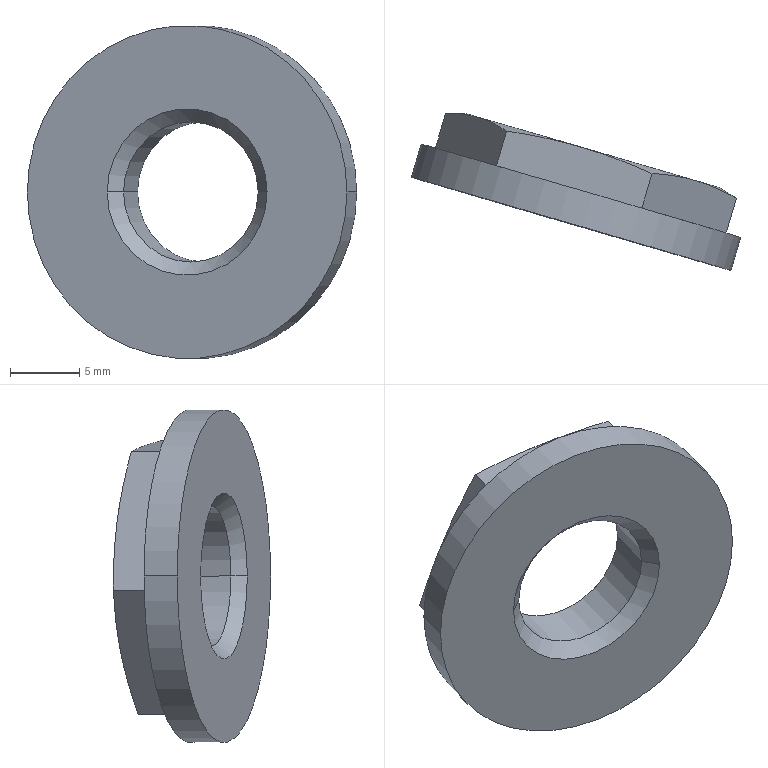Part | SolidWorks | features BaseBody 1 | 1 solid | 24 faces | box 23.74 x 11.323 x 24 mm | volume 1594 mm3 | cone 11 | plane 9 | cylinder 4 | commonest cylinder face diameters 10.106 x2 24 x2
STEP:
#1=CARTESIAN_POINT('',(-101.443,495.422,-24.879));
#2=VERTEX_POINT('',#1);
#3=CARTESIAN_POINT('',(-91.741,492.592,-24.879));
#4=VERTEX_POINT('',#3);
#5=CARTESIAN_POINT('',(-96.592,494.007,-24.879));
#6=DIRECTION('',(-0.28,-0.96,0.));
#7=DIRECTION('',(0.4011,-0.117,0.9085));
#8=AXIS2_PLACEMENT_3D('',#5,#6,#7);
#9=CIRCLE('',#8,5.053);
#10=EDGE_CURVE('',#2,#4,#9,.T.);
#11=ORIENTED_EDGE('',*,*,#10,.F.);
#12=CARTESIAN_POINT('',(-102.617,494.777,-24.879));
#13=VERTEX_POINT('',#12);
#14=CARTESIAN_POINT('',(-102.617,494.777,-24.879));
#15=DIRECTION('',(-0.8768,-0.4809,0.));
#16=VECTOR('',#15,1000.);
#17=LINE('',#14,#16);
#18=EDGE_CURVE('',#2,#13,#17,.T.);
#19=ORIENTED_EDGE('',*,*,#18,.T.);
#20=CARTESIAN_POINT('',(-91.097,491.418,-24.879));
#21=VERTEX_POINT('',#20);
#22=CARTESIAN_POINT('',(-96.857,493.098,-24.879));
#23=DIRECTION('',(0.28,0.96,0.));
#24=DIRECTION('',(0.96,-0.28,0.));
#25=AXIS2_PLACEMENT_3D('',#22,#23,#24);
#26=CIRCLE('',#25,6.);
#27=EDGE_CURVE('',#21,#13,#26,.T.);
#28=ORIENTED_EDGE('',*,*,#27,.F.);
#29=CARTESIAN_POINT('',(-91.097,491.418,-24.879));
#30=DIRECTION('',(0.4809,-0.8768,0.));
#31=VECTOR('',#30,1000.);
#32=LINE('',#29,#31);
#33=EDGE_CURVE('',#4,#21,#32,.T.);
#34=ORIENTED_EDGE('',*,*,#33,.F.);
#35=EDGE_LOOP('',(#11,#19,#28,#34));
#36=FACE_OUTER_BOUND('',#35,.T.);
#37=CARTESIAN_POINT('',(-96.857,493.098,-24.879));
#38=DIRECTION('',(-0.28,-0.96,0.));
#39=DIRECTION('',(0.96,-0.28,0.));
#40=AXIS2_PLACEMENT_3D('',#37,#38,#39);
#41=CONICAL_SURFACE('',#40,6.,0.7854);
#42=ADVANCED_FACE('',(#36),#41,.F.);
#43=CARTESIAN_POINT('',(-85.337,489.738,-24.879));
#44=VERTEX_POINT('',#43);
#45=CARTESIAN_POINT('',(-108.377,496.457,-24.879));
#46=VERTEX_POINT('',#45);
#47=CARTESIAN_POINT('',(-96.857,493.098,-24.879));
#48=DIRECTION('',(-0.28,-0.96,0.));
#49=DIRECTION('',(-0.96,0.28,0.));
#50=AXIS2_PLACEMENT_3D('',#47,#48,#49);
#51=CIRCLE('',#50,12.);
#52=EDGE_CURVE('',#44,#46,#51,.T.);
#53=ORIENTED_EDGE('',*,*,#52,.F.);
#54=CARTESIAN_POINT('',(-84.637,492.138,-24.879));
#55=VERTEX_POINT('',#54);
#56=CARTESIAN_POINT('',(-84.661,492.057,-24.879));
#57=DIRECTION('',(0.28,0.96,0.));
#58=VECTOR('',#57,1000.);
#59=LINE('',#56,#58);
#60=EDGE_CURVE('',#44,#55,#59,.T.);
#61=ORIENTED_EDGE('',*,*,#60,.T.);
#62=CARTESIAN_POINT('',(-107.677,498.857,-24.879));
#63=VERTEX_POINT('',#62);
#64=CARTESIAN_POINT('',(-96.157,495.498,-24.879));
#65=DIRECTION('',(-0.28,-0.96,0.));
#66=DIRECTION('',(-0.96,0.28,0.));
#67=AXIS2_PLACEMENT_3D('',#64,#65,#66);
#68=CIRCLE('',#67,12.);
#69=EDGE_CURVE('',#55,#63,#68,.T.);
#70=ORIENTED_EDGE('',*,*,#69,.T.);
#71=CARTESIAN_POINT('',(-107.701,498.776,-24.879));
#72=DIRECTION('',(0.28,0.96,0.));
#73=VECTOR('',#72,1000.);
#74=LINE('',#71,#73);
#75=EDGE_CURVE('',#46,#63,#74,.T.);
#76=ORIENTED_EDGE('',*,*,#75,.F.);
#77=EDGE_LOOP('',(#53,#61,#70,#76));
#78=FACE_OUTER_BOUND('',#77,.T.);
#79=CARTESIAN_POINT('',(-96.181,495.416,-24.879));
#80=DIRECTION('',(0.28,0.96,0.));
#81=DIRECTION('',(-0.96,0.28,0.));
#82=AXIS2_PLACEMENT_3D('',#79,#80,#81);
#83=CYLINDRICAL_SURFACE('',#82,12.);
#84=ADVANCED_FACE('',(#78),#83,.T.);
#85=ORIENTED_EDGE('',*,*,#10,.T.);
#86=CARTESIAN_POINT('',(-90.731,496.054,-24.879));
#87=VERTEX_POINT('',#86);
#88=CARTESIAN_POINT('',(-91.236,494.323,-24.879));
#89=DIRECTION('',(0.28,0.96,0.));
#90=VECTOR('',#89,1000.);
#91=LINE('',#88,#90);
#92=EDGE_CURVE('',#4,#87,#91,.T.);
#93=ORIENTED_EDGE('',*,*,#92,.T.);
#94=CARTESIAN_POINT('',(-100.433,498.883,-24.879));
#95=VERTEX_POINT('',#94);
#96=CARTESIAN_POINT('',(-95.582,497.469,-24.879));
#97=DIRECTION('',(-0.28,-0.96,0.));
#98=DIRECTION('',(-0.96,0.28,0.));
#99=AXIS2_PLACEMENT_3D('',#96,#97,#98);
#100=CIRCLE('',#99,5.053);
#101=EDGE_CURVE('',#95,#87,#100,.T.);
#102=ORIENTED_EDGE('',*,*,#101,.F.);
#103=CARTESIAN_POINT('',(-100.938,497.152,-24.879));
#104=DIRECTION('',(0.28,0.96,0.));
#105=VECTOR('',#104,1000.);
#106=LINE('',#103,#105);
#107=EDGE_CURVE('',#2,#95,#106,.T.);
#108=ORIENTED_EDGE('',*,*,#107,.F.);
#109=EDGE_LOOP('',(#85,#93,#102,#108));
#110=FACE_OUTER_BOUND('',#109,.T.);
#111=CARTESIAN_POINT('',(-96.087,495.738,-24.879));
#112=DIRECTION('',(0.28,0.96,0.));
#113=DIRECTION('',(-0.96,0.28,0.));
#114=AXIS2_PLACEMENT_3D('',#111,#112,#113);
#115=CYLINDRICAL_SURFACE('',#114,5.053);
#116=ADVANCED_FACE('',(#110),#115,.F.);
#117=ORIENTED_EDGE('',*,*,#101,.T.);
#118=CARTESIAN_POINT('',(-89.557,496.698,-24.879));
#119=VERTEX_POINT('',#118);
#120=CARTESIAN_POINT('',(-89.557,496.698,-24.879));
#121=DIRECTION('',(0.8768,0.4809,0.));
#122=VECTOR('',#121,1000.);
#123=LINE('',#120,#122);
#124=EDGE_CURVE('',#87,#119,#123,.T.);
#125=ORIENTED_EDGE('',*,*,#124,.T.);
#126=CARTESIAN_POINT('',(-101.077,500.058,-24.879));
#127=VERTEX_POINT('',#126);
#128=CARTESIAN_POINT('',(-95.317,498.378,-24.879));
#129=DIRECTION('',(-0.28,-0.96,0.));
#130=DIRECTION('',(-0.96,0.28,0.));
#131=AXIS2_PLACEMENT_3D('',#128,#129,#130);
#132=CIRCLE('',#131,6.);
#133=EDGE_CURVE('',#127,#119,#132,.T.);
#134=ORIENTED_EDGE('',*,*,#133,.F.);
#135=CARTESIAN_POINT('',(-101.077,500.058,-24.879));
#136=DIRECTION('',(-0.4809,0.8768,0.));
#137=VECTOR('',#136,1000.);
#138=LINE('',#135,#137);
#139=EDGE_CURVE('',#95,#127,#138,.T.);
#140=ORIENTED_EDGE('',*,*,#139,.F.);
#141=EDGE_LOOP('',(#117,#125,#134,#140));
#142=FACE_OUTER_BOUND('',#141,.T.);
#143=CARTESIAN_POINT('',(-95.317,498.378,-24.879));
#144=DIRECTION('',(0.28,0.96,0.));
#145=DIRECTION('',(-0.96,0.28,0.));
#146=AXIS2_PLACEMENT_3D('',#143,#144,#145);
#147=CONICAL_SURFACE('',#146,6.,0.7854);
#148=ADVANCED_FACE('',(#142),#147,.F.);
#149=CARTESIAN_POINT('',(-86.197,495.718,-24.879));
#150=VERTEX_POINT('',#149);
#151=CARTESIAN_POINT('',(-87.032,495.962,-28.848));
#152=VERTEX_POINT('',#151);
#153=CARTESIAN_POINT('',(-95.317,498.378,-24.879));
#154=DIRECTION('',(0.28,0.96,0.));
#155=DIRECTION('',(0.96,-0.28,0.));
#156=AXIS2_PLACEMENT_3D('',#153,#154,#155);
#157=CIRCLE('',#156,9.5);
#158=EDGE_CURVE('',#150,#152,#157,.T.);
#159=ORIENTED_EDGE('',*,*,#158,.F.);
#160=CARTESIAN_POINT('',(-85.351,495.204,-24.879));
#161=VERTEX_POINT('',#160);
#162=CARTESIAN_POINT('',(-84.889,494.924,-24.879));
#163=DIRECTION('',(0.8548,-0.5189,0.));
#164=VECTOR('',#163,1000.);
#165=LINE('',#162,#164);
#166=EDGE_CURVE('',#150,#161,#165,.T.);
#167=ORIENTED_EDGE('',*,*,#166,.T.);
#168=CARTESIAN_POINT('',(-85.351,495.204,-24.879));
#169=CARTESIAN_POINT('',(-85.887,495.53,-26.197));
#170=CARTESIAN_POINT('',(-86.445,495.791,-27.52));
#171=CARTESIAN_POINT('',(-87.032,495.962,-28.848));
#172=B_SPLINE_CURVE_WITH_KNOTS('',3,(#168,#169,#170,#171),.UNSPECIFIED.,.F.,.F.,(4,4),(0.001123,0.005499),.UNSPECIFIED.);
#173=EDGE_CURVE('',#161,#152,#172,.T.);
#174=ORIENTED_EDGE('',*,*,#173,.T.);
#175=EDGE_LOOP('',(#159,#167,#174));
#176=FACE_OUTER_BOUND('',#175,.T.);
#177=CARTESIAN_POINT('',(-95.428,497.998,-24.879));
#178=DIRECTION('',(-0.28,-0.96,0.));
#179=DIRECTION('',(0.96,-0.28,0.));
#180=AXIS2_PLACEMENT_3D('',#177,#178,#179);
#181=CONICAL_SURFACE('',#180,10.978,1.309);
#182=ADVANCED_FACE('',(#176),#181,.T.);
#183=ORIENTED_EDGE('',*,*,#27,.T.);
#184=CARTESIAN_POINT('',(-96.857,493.098,-24.879));
#185=DIRECTION('',(0.28,0.96,0.));
#186=DIRECTION('',(0.96,-0.28,0.));
#187=AXIS2_PLACEMENT_3D('',#184,#185,#186);
#188=CIRCLE('',#187,6.);
#189=EDGE_CURVE('',#13,#21,#188,.T.);
#190=ORIENTED_EDGE('',*,*,#189,.T.);
#191=EDGE_LOOP('',(#183,#190));
#192=FACE_BOUND('',#191,.T.);
#193=CARTESIAN_POINT('',(-96.857,493.098,-24.879));
#194=DIRECTION('',(-0.28,-0.96,0.));
#195=DIRECTION('',(-0.96,0.28,0.));
#196=AXIS2_PLACEMENT_3D('',#193,#194,#195);
#197=CIRCLE('',#196,12.);
#198=EDGE_CURVE('',#46,#44,#197,.T.);
#199=ORIENTED_EDGE('',*,*,#198,.T.);
#200=ORIENTED_EDGE('',*,*,#52,.T.);
#201=EDGE_LOOP('',(#199,#200));
#202=FACE_OUTER_BOUND('',#201,.T.);
#203=CARTESIAN_POINT('',(-93.247,492.045,-16.702));
#204=DIRECTION('',(-0.28,-0.96,0.));
#205=DIRECTION('',(0.96,-0.28,0.));
#206=AXIS2_PLACEMENT_3D('',#203,#204,#205);
#207=PLANE('',#206);
#208=ADVANCED_FACE('',(#192,#202),#207,.T.);
#209=ORIENTED_EDGE('',*,*,#18,.F.);
#210=CARTESIAN_POINT('',(-96.592,494.007,-24.879));
#211=DIRECTION('',(-0.28,-0.96,0.));
#212=DIRECTION('',(0.4011,-0.117,0.9085));
#213=AXIS2_PLACEMENT_3D('',#210,#211,#212);
#214=CIRCLE('',#213,5.053);
#215=EDGE_CURVE('',#4,#2,#214,.T.);
#216=ORIENTED_EDGE('',*,*,#215,.F.);
#217=ORIENTED_EDGE('',*,*,#33,.T.);
#218=ORIENTED_EDGE('',*,*,#189,.F.);
#219=EDGE_LOOP('',(#209,#216,#217,#218));
#220=FACE_OUTER_BOUND('',#219,.T.);
#221=CARTESIAN_POINT('',(-96.857,493.098,-24.879));
#222=DIRECTION('',(-0.28,-0.96,0.));
#223=DIRECTION('',(0.96,-0.28,0.));
#224=AXIS2_PLACEMENT_3D('',#221,#222,#223);
#225=CONICAL_SURFACE('',#224,6.,0.7854);
#226=ADVANCED_FACE('',(#220),#225,.F.);
#227=ORIENTED_EDGE('',*,*,#60,.F.);
#228=ORIENTED_EDGE('',*,*,#198,.F.);
#229=ORIENTED_EDGE('',*,*,#75,.T.);
#230=CARTESIAN_POINT('',(-96.157,495.498,-24.879));
#231=DIRECTION('',(-0.28,-0.96,0.));
#232=DIRECTION('',(-0.96,0.28,0.));
#233=AXIS2_PLACEMENT_3D('',#230,#231,#232);
#234=CIRCLE('',#233,12.);
#235=EDGE_CURVE('',#63,#55,#234,.T.);
#236=ORIENTED_EDGE('',*,*,#235,.T.);
#237=EDGE_LOOP('',(#227,#228,#229,#236));
#238=FACE_OUTER_BOUND('',#237,.T.);
#239=CARTESIAN_POINT('',(-96.181,495.416,-24.879));
#240=DIRECTION('',(0.28,0.96,0.));
#241=DIRECTION('',(-0.96,0.28,0.));
#242=AXIS2_PLACEMENT_3D('',#239,#240,#241);
#243=CYLINDRICAL_SURFACE('',#242,12.);
#244=ADVANCED_FACE('',(#238),#243,.T.);
#245=ORIENTED_EDGE('',*,*,#92,.F.);
#246=ORIENTED_EDGE('',*,*,#215,.T.);
#247=ORIENTED_EDGE('',*,*,#107,.T.);
#248=CARTESIAN_POINT('',(-95.582,497.469,-24.879));
#249=DIRECTION('',(-0.28,-0.96,0.));
#250=DIRECTION('',(-0.96,0.28,0.));
#251=AXIS2_PLACEMENT_3D('',#248,#249,#250);
#252=CIRCLE('',#251,5.053);
#253=EDGE_CURVE('',#87,#95,#252,.T.);
#254=ORIENTED_EDGE('',*,*,#253,.F.);
#255=EDGE_LOOP('',(#245,#246,#247,#254));
#256=FACE_OUTER_BOUND('',#255,.T.);
#257=CARTESIAN_POINT('',(-96.087,495.738,-24.879));
#258=DIRECTION('',(0.28,0.96,0.));
#259=DIRECTION('',(-0.96,0.28,0.));
#260=AXIS2_PLACEMENT_3D('',#257,#258,#259);
#261=CYLINDRICAL_SURFACE('',#260,5.053);
#262=ADVANCED_FACE('',(#256),#261,.F.);
#263=ORIENTED_EDGE('',*,*,#235,.F.);
#264=ORIENTED_EDGE('',*,*,#69,.F.);
#265=EDGE_LOOP('',(#263,#264));
#266=FACE_OUTER_BOUND('',#265,.T.);
#267=CARTESIAN_POINT('',(-90.072,493.723,-33.832));
#268=VERTEX_POINT('',#267);
#269=CARTESIAN_POINT('',(-85.671,492.44,-23.865));
#270=VERTEX_POINT('',#269);
#271=CARTESIAN_POINT('',(-90.072,493.723,-33.832));
#272=DIRECTION('',(0.4011,-0.117,0.9085));
#273=VECTOR('',#272,1000.);
#274=LINE('',#271,#273);
#275=EDGE_CURVE('',#268,#270,#274,.T.);
#276=ORIENTED_EDGE('',*,*,#275,.T.);
#277=CARTESIAN_POINT('',(-91.757,494.215,-14.913));
#278=VERTEX_POINT('',#277);
#279=CARTESIAN_POINT('',(-85.671,492.44,-23.865));
#280=DIRECTION('',(-0.5548,0.1618,0.8161));
#281=VECTOR('',#280,1000.);
#282=LINE('',#279,#281);
#283=EDGE_CURVE('',#270,#278,#282,.T.);
#284=ORIENTED_EDGE('',*,*,#283,.T.);
#285=CARTESIAN_POINT('',(-102.243,497.272,-15.926));
#286=VERTEX_POINT('',#285);
#287=CARTESIAN_POINT('',(-91.757,494.215,-14.913));
#288=DIRECTION('',(-0.9559,0.2788,-0.0924));
#289=VECTOR('',#288,1000.);
#290=LINE('',#287,#289);
#291=EDGE_CURVE('',#278,#286,#290,.T.);
#292=ORIENTED_EDGE('',*,*,#291,.T.);
#293=CARTESIAN_POINT('',(-106.643,498.556,-25.892));
#294=VERTEX_POINT('',#293);
#295=CARTESIAN_POINT('',(-102.243,497.272,-15.926));
#296=DIRECTION('',(-0.4011,0.117,-0.9085));
#297=VECTOR('',#296,1000.);
#298=LINE('',#295,#297);
#299=EDGE_CURVE('',#286,#294,#298,.T.);
#300=ORIENTED_EDGE('',*,*,#299,.T.);
#301=CARTESIAN_POINT('',(-100.558,496.781,-34.845));
#302=VERTEX_POINT('',#301);
#303=CARTESIAN_POINT('',(-106.643,498.556,-25.892));
#304=DIRECTION('',(0.5548,-0.1618,-0.8161));
#305=VECTOR('',#304,1000.);
#306=LINE('',#303,#305);
#307=EDGE_CURVE('',#294,#302,#306,.T.);
#308=ORIENTED_EDGE('',*,*,#307,.T.);
#309=CARTESIAN_POINT('',(-100.558,496.781,-34.845));
#310=DIRECTION('',(0.9559,-0.2788,0.0924));
#311=VECTOR('',#310,1000.);
#312=LINE('',#309,#311);
#313=EDGE_CURVE('',#302,#268,#312,.T.);
#314=ORIENTED_EDGE('',*,*,#313,.T.);
#315=EDGE_LOOP('',(#276,#284,#292,#300,#308,#314));
#316=FACE_BOUND('',#315,.T.);
#317=CARTESIAN_POINT('',(-96.157,495.498,-24.879));
#318=DIRECTION('',(0.28,0.96,0.));
#319=DIRECTION('',(-0.96,0.28,0.));
#320=AXIS2_PLACEMENT_3D('',#317,#318,#319);
#321=PLANE('',#320);
#322=ADVANCED_FACE('',(#266,#316),#321,.T.);
#323=ORIENTED_EDGE('',*,*,#124,.F.);
#324=ORIENTED_EDGE('',*,*,#253,.T.);
#325=ORIENTED_EDGE('',*,*,#139,.T.);
#326=CARTESIAN_POINT('',(-95.317,498.378,-24.879));
#327=DIRECTION('',(-0.28,-0.96,0.));
#328=DIRECTION('',(-0.96,0.28,0.));
#329=AXIS2_PLACEMENT_3D('',#326,#327,#328);
#330=CIRCLE('',#329,6.);
#331=EDGE_CURVE('',#119,#127,#330,.T.);
#332=ORIENTED_EDGE('',*,*,#331,.F.);
#333=EDGE_LOOP('',(#323,#324,#325,#332));
#334=FACE_OUTER_BOUND('',#333,.T.);
#335=CARTESIAN_POINT('',(-95.317,498.378,-24.879));
#336=DIRECTION('',(0.28,0.96,0.));
#337=DIRECTION('',(-0.96,0.28,0.));
#338=AXIS2_PLACEMENT_3D('',#335,#336,#337);
#339=CONICAL_SURFACE('',#338,6.,0.7854);
#340=ADVANCED_FACE('',(#334),#339,.F.);
#341=CARTESIAN_POINT('',(-91.027,496.717,-14.913));
#342=VERTEX_POINT('',#341);
#343=CARTESIAN_POINT('',(-91.757,494.215,-14.913));
#344=DIRECTION('',(0.28,0.96,0.));
#345=VECTOR('',#344,1000.);
#346=LINE('',#343,#345);
#347=EDGE_CURVE('',#278,#342,#346,.T.);
#348=ORIENTED_EDGE('',*,*,#347,.F.);
#349=ORIENTED_EDGE('',*,*,#283,.F.);
#350=CARTESIAN_POINT('',(-84.942,494.942,-23.865));
#351=VERTEX_POINT('',#350);
#352=CARTESIAN_POINT('',(-84.942,494.942,-23.865));
#353=DIRECTION('',(-0.28,-0.96,0.));
#354=VECTOR('',#353,1000.);
#355=LINE('',#352,#354);
#356=EDGE_CURVE('',#351,#270,#355,.T.);
#357=ORIENTED_EDGE('',*,*,#356,.F.);
#358=CARTESIAN_POINT('',(-87.874,496.207,-19.389));
#359=VERTEX_POINT('',#358);
#360=CARTESIAN_POINT('',(-87.874,496.207,-19.389));
#361=CARTESIAN_POINT('',(-87.364,496.059,-20.139));
#362=CARTESIAN_POINT('',(-86.866,495.876,-20.887));
#363=CARTESIAN_POINT('',(-85.89,495.449,-22.379));
#364=CARTESIAN_POINT('',(-85.412,495.206,-23.123));
#365=CARTESIAN_POINT('',(-84.942,494.942,-23.865));
#366=B_SPLINE_CURVE_WITH_KNOTS('',3,(#360,#361,#362,#363,#364,#365),.UNSPECIFIED.,.F.,.F.,(4,2,4),(0.,0.002749,0.005499),.UNSPECIFIED.);
#367=EDGE_CURVE('',#359,#351,#366,.T.);
#368=ORIENTED_EDGE('',*,*,#367,.F.);
#369=CARTESIAN_POINT('',(-91.027,496.717,-14.913));
#370=CARTESIAN_POINT('',(-90.488,496.686,-15.656));
#371=CARTESIAN_POINT('',(-89.955,496.634,-16.4));
#372=CARTESIAN_POINT('',(-88.902,496.469,-17.891));
#373=CARTESIAN_POINT('',(-88.384,496.356,-18.639));
#374=CARTESIAN_POINT('',(-87.874,496.207,-19.389));
#375=B_SPLINE_CURVE_WITH_KNOTS('',3,(#369,#370,#371,#372,#373,#374),.UNSPECIFIED.,.F.,.F.,(4,2,4),(0.,0.002749,0.005499),.UNSPECIFIED.);
#376=EDGE_CURVE('',#342,#359,#375,.T.);
#377=ORIENTED_EDGE('',*,*,#376,.F.);
#378=EDGE_LOOP('',(#348,#349,#357,#368,#377));
#379=FACE_OUTER_BOUND('',#378,.T.);
#380=CARTESIAN_POINT('',(-91.757,494.215,-14.913));
#381=DIRECTION('',(-0.7835,0.2285,-0.5779));
#382=DIRECTION('',(-0.5936,0.,0.8048));
#383=AXIS2_PLACEMENT_3D('',#380,#381,#382);
#384=PLANE('',#383);
#385=ADVANCED_FACE('',(#379),#384,.F.);
#386=ORIENTED_EDGE('',*,*,#275,.F.);
#387=CARTESIAN_POINT('',(-89.342,496.225,-33.832));
#388=VERTEX_POINT('',#387);
#389=CARTESIAN_POINT('',(-89.342,496.225,-33.832));
#390=DIRECTION('',(-0.28,-0.96,0.));
#391=VECTOR('',#390,1000.);
#392=LINE('',#389,#391);
#393=EDGE_CURVE('',#388,#268,#392,.T.);
#394=ORIENTED_EDGE('',*,*,#393,.F.);
#395=CARTESIAN_POINT('',(-87.032,495.962,-28.848));
#396=CARTESIAN_POINT('',(-87.4,496.069,-29.683));
#397=CARTESIAN_POINT('',(-87.778,496.141,-30.516));
#398=CARTESIAN_POINT('',(-88.549,496.224,-32.176));
#399=CARTESIAN_POINT('',(-88.943,496.236,-33.005));
#400=CARTESIAN_POINT('',(-89.342,496.225,-33.832));
#401=B_SPLINE_CURVE_WITH_KNOTS('',3,(#395,#396,#397,#398,#399,#400),.UNSPECIFIED.,.F.,.F.,(4,2,4),(0.,0.002749,0.005499),.UNSPECIFIED.);
#402=EDGE_CURVE('',#152,#388,#401,.T.);
#403=ORIENTED_EDGE('',*,*,#402,.F.);
#404=ORIENTED_EDGE('',*,*,#173,.F.);
#405=CARTESIAN_POINT('',(-84.942,494.942,-23.865));
#406=CARTESIAN_POINT('',(-85.077,495.033,-24.203));
#407=CARTESIAN_POINT('',(-85.213,495.121,-24.541));
#408=CARTESIAN_POINT('',(-85.351,495.204,-24.879));
#409=B_SPLINE_CURVE_WITH_KNOTS('',3,(#405,#406,#407,#408),.UNSPECIFIED.,.F.,.F.,(4,4),(0.,0.001123),.UNSPECIFIED.);
#410=EDGE_CURVE('',#351,#161,#409,.T.);
#411=ORIENTED_EDGE('',*,*,#410,.F.);
#412=ORIENTED_EDGE('',*,*,#356,.T.);
#413=EDGE_LOOP('',(#386,#394,#403,#404,#411,#412));
#414=FACE_OUTER_BOUND('',#413,.T.);
#415=CARTESIAN_POINT('',(-85.671,492.44,-23.865));
#416=DIRECTION('',(-0.8722,0.2543,0.4178));
#417=DIRECTION('',(0.4321,0.,0.9018));
#418=AXIS2_PLACEMENT_3D('',#415,#416,#417);
#419=PLANE('',#418);
#420=ADVANCED_FACE('',(#414),#419,.F.);
#421=ORIENTED_EDGE('',*,*,#313,.F.);
#422=CARTESIAN_POINT('',(-99.828,499.283,-34.845));
#423=VERTEX_POINT('',#422);
#424=CARTESIAN_POINT('',(-99.828,499.283,-34.845));
#425=DIRECTION('',(-0.28,-0.96,0.));
#426=VECTOR('',#425,1000.);
#427=LINE('',#424,#426);
#428=EDGE_CURVE('',#423,#302,#427,.T.);
#429=ORIENTED_EDGE('',*,*,#428,.F.);
#430=CARTESIAN_POINT('',(-94.475,498.132,-34.338));
#431=VERTEX_POINT('',#430);
#432=CARTESIAN_POINT('',(-94.475,498.132,-34.338));
#433=CARTESIAN_POINT('',(-95.353,498.388,-34.423));
#434=CARTESIAN_POINT('',(-96.239,498.609,-34.508));
#435=CARTESIAN_POINT('',(-98.024,498.988,-34.677));
#436=CARTESIAN_POINT('',(-98.924,499.146,-34.761));
#437=CARTESIAN_POINT('',(-99.828,499.283,-34.845));
#438=B_SPLINE_CURVE_WITH_KNOTS('',3,(#432,#433,#434,#435,#436,#437),.UNSPECIFIED.,.F.,.F.,(4,2,4),(0.,0.002749,0.005499),.UNSPECIFIED.);
#439=EDGE_CURVE('',#431,#423,#438,.T.);
#440=ORIENTED_EDGE('',*,*,#439,.F.);
#441=CARTESIAN_POINT('',(-89.342,496.225,-33.832));
#442=CARTESIAN_POINT('',(-90.178,496.596,-33.916));
#443=CARTESIAN_POINT('',(-91.021,496.945,-34.));
#444=CARTESIAN_POINT('',(-92.731,497.586,-34.169));
#445=CARTESIAN_POINT('',(-93.596,497.876,-34.253));
#446=CARTESIAN_POINT('',(-94.475,498.132,-34.338));
#447=B_SPLINE_CURVE_WITH_KNOTS('',3,(#441,#442,#443,#444,#445,#446),.UNSPECIFIED.,.F.,.F.,(4,2,4),(0.,0.002749,0.005499),.UNSPECIFIED.);
#448=EDGE_CURVE('',#388,#431,#447,.T.);
#449=ORIENTED_EDGE('',*,*,#448,.F.);
#450=ORIENTED_EDGE('',*,*,#393,.T.);
#451=EDGE_LOOP('',(#421,#429,#440,#449,#450));
#452=FACE_OUTER_BOUND('',#451,.T.);
#453=CARTESIAN_POINT('',(-90.072,493.723,-33.832));
#454=DIRECTION('',(-0.0887,0.02587,0.9957));
#455=DIRECTION('',(0.9961,0.,0.08873));
#456=AXIS2_PLACEMENT_3D('',#453,#454,#455);
#457=PLANE('',#456);
#458=ADVANCED_FACE('',(#452),#457,.F.);
#459=ORIENTED_EDGE('',*,*,#307,.F.);
#460=CARTESIAN_POINT('',(-105.914,501.058,-25.892));
#461=VERTEX_POINT('',#460);
#462=CARTESIAN_POINT('',(-105.914,501.058,-25.892));
#463=DIRECTION('',(-0.28,-0.96,0.));
#464=VECTOR('',#463,1000.);
#465=LINE('',#462,#464);
#466=EDGE_CURVE('',#461,#294,#465,.T.);
#467=ORIENTED_EDGE('',*,*,#466,.F.);
#468=CARTESIAN_POINT('',(-102.76,500.548,-30.369));
#469=VERTEX_POINT('',#468);
#470=CARTESIAN_POINT('',(-102.76,500.548,-30.369));
#471=CARTESIAN_POINT('',(-103.27,500.697,-29.619));
#472=CARTESIAN_POINT('',(-103.789,500.81,-28.871));
#473=CARTESIAN_POINT('',(-104.841,500.975,-27.379));
#474=CARTESIAN_POINT('',(-105.375,501.027,-26.635));
#475=CARTESIAN_POINT('',(-105.914,501.058,-25.892));
#476=B_SPLINE_CURVE_WITH_KNOTS('',3,(#470,#471,#472,#473,#474,#475),.UNSPECIFIED.,.F.,.F.,(4,2,4),(0.,0.002749,0.005499),.UNSPECIFIED.);
#477=EDGE_CURVE('',#469,#461,#476,.T.);
#478=ORIENTED_EDGE('',*,*,#477,.F.);
#479=CARTESIAN_POINT('',(-99.828,499.283,-34.845));
#480=CARTESIAN_POINT('',(-100.299,499.547,-34.102));
#481=CARTESIAN_POINT('',(-100.777,499.79,-33.358));
#482=CARTESIAN_POINT('',(-101.753,500.217,-31.866));
#483=CARTESIAN_POINT('',(-102.251,500.4,-31.119));
#484=CARTESIAN_POINT('',(-102.76,500.548,-30.369));
#485=B_SPLINE_CURVE_WITH_KNOTS('',3,(#479,#480,#481,#482,#483,#484),.UNSPECIFIED.,.F.,.F.,(4,2,4),(0.,0.002749,0.005499),.UNSPECIFIED.);
#486=EDGE_CURVE('',#423,#469,#485,.T.);
#487=ORIENTED_EDGE('',*,*,#486,.F.);
#488=ORIENTED_EDGE('',*,*,#428,.T.);
#489=EDGE_LOOP('',(#459,#467,#478,#487,#488));
#490=FACE_OUTER_BOUND('',#489,.T.);
#491=CARTESIAN_POINT('',(-100.558,496.781,-34.845));
#492=DIRECTION('',(0.7835,-0.2285,0.5779));
#493=DIRECTION('',(0.5936,0.,-0.8048));
#494=AXIS2_PLACEMENT_3D('',#491,#492,#493);
#495=PLANE('',#494);
#496=ADVANCED_FACE('',(#490),#495,.F.);
#497=ORIENTED_EDGE('',*,*,#466,.T.);
#498=ORIENTED_EDGE('',*,*,#299,.F.);
#499=CARTESIAN_POINT('',(-101.513,499.774,-15.926));
#500=VERTEX_POINT('',#499);
#501=CARTESIAN_POINT('',(-101.513,499.774,-15.926));
#502=DIRECTION('',(-0.28,-0.96,0.));
#503=VECTOR('',#502,1000.);
#504=LINE('',#501,#503);
#505=EDGE_CURVE('',#500,#286,#504,.T.);
#506=ORIENTED_EDGE('',*,*,#505,.F.);
#507=CARTESIAN_POINT('',(-103.603,500.794,-20.909));
#508=VERTEX_POINT('',#507);
#509=CARTESIAN_POINT('',(-103.603,500.794,-20.909));
#510=CARTESIAN_POINT('',(-103.235,500.687,-20.075));
#511=CARTESIAN_POINT('',(-102.877,500.545,-19.242));
#512=CARTESIAN_POINT('',(-102.182,500.2,-17.581));
#513=CARTESIAN_POINT('',(-101.844,499.998,-16.753));
#514=CARTESIAN_POINT('',(-101.513,499.774,-15.926));
#515=B_SPLINE_CURVE_WITH_KNOTS('',3,(#509,#510,#511,#512,#513,#514),.UNSPECIFIED.,.F.,.F.,(4,2,4),(0.,0.002749,0.005499),.UNSPECIFIED.);
#516=EDGE_CURVE('',#508,#500,#515,.T.);
#517=ORIENTED_EDGE('',*,*,#516,.F.);
#518=CARTESIAN_POINT('',(-105.914,501.058,-25.892));
#519=CARTESIAN_POINT('',(-105.514,501.068,-25.066));
#520=CARTESIAN_POINT('',(-105.121,501.057,-24.237));
#521=CARTESIAN_POINT('',(-104.349,500.974,-22.577));
#522=CARTESIAN_POINT('',(-103.972,500.902,-21.744));
#523=CARTESIAN_POINT('',(-103.603,500.794,-20.909));
#524=B_SPLINE_CURVE_WITH_KNOTS('',3,(#518,#519,#520,#521,#522,#523),.UNSPECIFIED.,.F.,.F.,(4,2,4),(0.,0.002749,0.005499),.UNSPECIFIED.);
#525=EDGE_CURVE('',#461,#508,#524,.T.);
#526=ORIENTED_EDGE('',*,*,#525,.F.);
#527=EDGE_LOOP('',(#497,#498,#506,#517,#526));
#528=FACE_OUTER_BOUND('',#527,.T.);
#529=CARTESIAN_POINT('',(-106.643,498.556,-25.892));
#530=DIRECTION('',(0.8722,-0.2543,-0.4178));
#531=DIRECTION('',(-0.4321,0.,-0.9018));
#532=AXIS2_PLACEMENT_3D('',#529,#530,#531);
#533=PLANE('',#532);
#534=ADVANCED_FACE('',(#528),#533,.F.);
#535=ORIENTED_EDGE('',*,*,#505,.T.);
#536=ORIENTED_EDGE('',*,*,#291,.F.);
#537=ORIENTED_EDGE('',*,*,#347,.T.);
#538=CARTESIAN_POINT('',(-96.16,498.624,-15.42));
#539=VERTEX_POINT('',#538);
#540=CARTESIAN_POINT('',(-96.16,498.624,-15.42));
#541=CARTESIAN_POINT('',(-95.282,498.367,-15.335));
#542=CARTESIAN_POINT('',(-94.416,498.077,-15.25));
#543=CARTESIAN_POINT('',(-92.707,497.437,-15.081));
#544=CARTESIAN_POINT('',(-91.863,497.087,-14.997));
#545=CARTESIAN_POINT('',(-91.027,496.717,-14.913));
#546=B_SPLINE_CURVE_WITH_KNOTS('',3,(#540,#541,#542,#543,#544,#545),.UNSPECIFIED.,.F.,.F.,(4,2,4),(0.,0.002749,0.005499),.UNSPECIFIED.);
#547=EDGE_CURVE('',#539,#342,#546,.T.);
#548=ORIENTED_EDGE('',*,*,#547,.F.);
#549=CARTESIAN_POINT('',(-101.513,499.774,-15.926));
#550=CARTESIAN_POINT('',(-100.609,499.638,-15.842));
#551=CARTESIAN_POINT('',(-99.71,499.479,-15.758));
#552=CARTESIAN_POINT('',(-97.924,499.1,-15.589));
#553=CARTESIAN_POINT('',(-97.038,498.88,-15.504));
#554=CARTESIAN_POINT('',(-96.16,498.624,-15.42));
#555=B_SPLINE_CURVE_WITH_KNOTS('',3,(#549,#550,#551,#552,#553,#554),.UNSPECIFIED.,.F.,.F.,(4,2,4),(0.,0.002749,0.005499),.UNSPECIFIED.);
#556=EDGE_CURVE('',#500,#539,#555,.T.);
#557=ORIENTED_EDGE('',*,*,#556,.F.);
#558=EDGE_LOOP('',(#535,#536,#537,#548,#557));
#559=FACE_OUTER_BOUND('',#558,.T.);
#560=CARTESIAN_POINT('',(-102.243,497.272,-15.926));
#561=DIRECTION('',(0.0887,-0.02587,-0.9957));
#562=DIRECTION('',(-0.9961,0.,-0.08873));
#563=AXIS2_PLACEMENT_3D('',#560,#561,#562);
#564=PLANE('',#563);
#565=ADVANCED_FACE('',(#559),#564,.F.);
#566=CARTESIAN_POINT('',(-95.317,498.378,-24.879));
#567=DIRECTION('',(0.28,0.96,0.));
#568=DIRECTION('',(0.96,-0.28,0.));
#569=AXIS2_PLACEMENT_3D('',#566,#567,#568);
#570=CIRCLE('',#569,9.5);
#571=EDGE_CURVE('',#431,#469,#570,.T.);
#572=ORIENTED_EDGE('',*,*,#571,.T.);
#573=CARTESIAN_POINT('',(-95.317,498.378,-24.879));
#574=DIRECTION('',(0.28,0.96,0.));
#575=DIRECTION('',(0.96,-0.28,0.));
#576=AXIS2_PLACEMENT_3D('',#573,#574,#575);
#577=CIRCLE('',#576,9.5);
#578=EDGE_CURVE('',#469,#508,#577,.T.);
#579=ORIENTED_EDGE('',*,*,#578,.T.);
#580=CARTESIAN_POINT('',(-95.317,498.378,-24.879));
#581=DIRECTION('',(0.28,0.96,0.));
#582=DIRECTION('',(0.96,-0.28,0.));
#583=AXIS2_PLACEMENT_3D('',#580,#581,#582);
#584=CIRCLE('',#583,9.5);
#585=EDGE_CURVE('',#508,#539,#584,.T.);
#586=ORIENTED_EDGE('',*,*,#585,.T.);
#587=CARTESIAN_POINT('',(-95.317,498.378,-24.879));
#588=DIRECTION('',(0.28,0.96,0.));
#589=DIRECTION('',(0.96,-0.28,0.));
#590=AXIS2_PLACEMENT_3D('',#587,#588,#589);
#591=CIRCLE('',#590,9.5);
#592=EDGE_CURVE('',#539,#359,#591,.T.);
#593=ORIENTED_EDGE('',*,*,#592,.T.);
#594=CARTESIAN_POINT('',(-95.317,498.378,-24.879));
#595=DIRECTION('',(0.28,0.96,0.));
#596=DIRECTION('',(0.96,-0.28,0.));
#597=AXIS2_PLACEMENT_3D('',#594,#595,#596);
#598=CIRCLE('',#597,9.5);
#599=EDGE_CURVE('',#359,#150,#598,.T.);
#600=ORIENTED_EDGE('',*,*,#599,.T.);
#601=ORIENTED_EDGE('',*,*,#158,.T.);
#602=CARTESIAN_POINT('',(-95.317,498.378,-24.879));
#603=DIRECTION('',(0.28,0.96,0.));
#604=DIRECTION('',(0.96,-0.28,0.));
#605=AXIS2_PLACEMENT_3D('',#602,#603,#604);
#606=CIRCLE('',#605,9.5);
#607=EDGE_CURVE('',#152,#431,#606,.T.);
#608=ORIENTED_EDGE('',*,*,#607,.T.);
#609=EDGE_LOOP('',(#572,#579,#586,#593,#600,#601,#608));
#610=FACE_OUTER_BOUND('',#609,.T.);
#611=ORIENTED_EDGE('',*,*,#133,.T.);
#612=ORIENTED_EDGE('',*,*,#331,.T.);
#613=EDGE_LOOP('',(#611,#612));
#614=FACE_BOUND('',#613,.T.);
#615=CARTESIAN_POINT('',(-92.209,497.471,-17.838));
#616=DIRECTION('',(0.28,0.96,0.));
#617=DIRECTION('',(-0.96,0.28,0.));
#618=AXIS2_PLACEMENT_3D('',#615,#616,#617);
#619=PLANE('',#618);
#620=ADVANCED_FACE('',(#610,#614),#619,.T.);
#621=ORIENTED_EDGE('',*,*,#547,.T.);
#622=ORIENTED_EDGE('',*,*,#376,.T.);
#623=ORIENTED_EDGE('',*,*,#592,.F.);
#624=EDGE_LOOP('',(#621,#622,#623));
#625=FACE_OUTER_BOUND('',#624,.T.);
#626=CARTESIAN_POINT('',(-95.428,497.998,-24.879));
#627=DIRECTION('',(-0.28,-0.96,0.));
#628=DIRECTION('',(0.96,-0.28,0.));
#629=AXIS2_PLACEMENT_3D('',#626,#627,#628);
#630=CONICAL_SURFACE('',#629,10.978,1.309);
#631=ADVANCED_FACE('',(#625),#630,.T.);
#632=ORIENTED_EDGE('',*,*,#166,.F.);
#633=ORIENTED_EDGE('',*,*,#599,.F.);
#634=ORIENTED_EDGE('',*,*,#367,.T.);
#635=ORIENTED_EDGE('',*,*,#410,.T.);
#636=EDGE_LOOP('',(#632,#633,#634,#635));
#637=FACE_OUTER_BOUND('',#636,.T.);
#638=CARTESIAN_POINT('',(-95.428,497.998,-24.879));
#639=DIRECTION('',(-0.28,-0.96,0.));
#640=DIRECTION('',(0.96,-0.28,0.));
#641=AXIS2_PLACEMENT_3D('',#638,#639,#640);
#642=CONICAL_SURFACE('',#641,10.978,1.309);
#643=ADVANCED_FACE('',(#637),#642,.T.);
#644=ORIENTED_EDGE('',*,*,#607,.F.);
#645=ORIENTED_EDGE('',*,*,#402,.T.);
#646=ORIENTED_EDGE('',*,*,#448,.T.);
#647=EDGE_LOOP('',(#644,#645,#646));
#648=FACE_OUTER_BOUND('',#647,.T.);
#649=CARTESIAN_POINT('',(-95.428,497.998,-24.879));
#650=DIRECTION('',(-0.28,-0.96,0.));
#651=DIRECTION('',(0.96,-0.28,0.));
#652=AXIS2_PLACEMENT_3D('',#649,#650,#651);
#653=CONICAL_SURFACE('',#652,10.978,1.309);
#654=ADVANCED_FACE('',(#648),#653,.T.);
#655=ORIENTED_EDGE('',*,*,#571,.F.);
#656=ORIENTED_EDGE('',*,*,#439,.T.);
#657=ORIENTED_EDGE('',*,*,#486,.T.);
#658=EDGE_LOOP('',(#655,#656,#657));
#659=FACE_OUTER_BOUND('',#658,.T.);
#660=CARTESIAN_POINT('',(-95.428,497.998,-24.879));
#661=DIRECTION('',(-0.28,-0.96,0.));
#662=DIRECTION('',(0.96,-0.28,0.));
#663=AXIS2_PLACEMENT_3D('',#660,#661,#662);
#664=CONICAL_SURFACE('',#663,10.978,1.309);
#665=ADVANCED_FACE('',(#659),#664,.T.);
#666=ORIENTED_EDGE('',*,*,#578,.F.);
#667=ORIENTED_EDGE('',*,*,#477,.T.);
#668=ORIENTED_EDGE('',*,*,#525,.T.);
#669=EDGE_LOOP('',(#666,#667,#668));
#670=FACE_OUTER_BOUND('',#669,.T.);
#671=CARTESIAN_POINT('',(-95.428,497.998,-24.879));
#672=DIRECTION('',(-0.28,-0.96,0.));
#673=DIRECTION('',(0.96,-0.28,0.));
#674=AXIS2_PLACEMENT_3D('',#671,#672,#673);
#675=CONICAL_SURFACE('',#674,10.978,1.309);
#676=ADVANCED_FACE('',(#670),#675,.T.);
#677=ORIENTED_EDGE('',*,*,#516,.T.);
#678=ORIENTED_EDGE('',*,*,#556,.T.);
#679=ORIENTED_EDGE('',*,*,#585,.F.);
#680=EDGE_LOOP('',(#677,#678,#679));
#681=FACE_OUTER_BOUND('',#680,.T.);
#682=CARTESIAN_POINT('',(-95.428,497.998,-24.879));
#683=DIRECTION('',(-0.28,-0.96,0.));
#684=DIRECTION('',(0.96,-0.28,0.));
#685=AXIS2_PLACEMENT_3D('',#682,#683,#684);
#686=CONICAL_SURFACE('',#685,10.978,1.309);
#687=ADVANCED_FACE('',(#681),#686,.T.);
#688=CLOSED_SHELL('',(#42,#84,#116,#148,#182,#208,#226,#244,#262,#322,#340,#385,#420,#458,#496,#534,#565,#620,#631,#643,#654,#665,#676,#687));
#689=MANIFOLD_SOLID_BREP('',#688);
#690=CARTESIAN_POINT('',(0.,0.,0.));
#691=DIRECTION('',(0.,0.,1.));
#692=DIRECTION('',(1.,0.,0.));
#693=AXIS2_PLACEMENT_3D('',#690,#691,#692);
#694=(LENGTH_UNIT()NAMED_UNIT(*)SI_UNIT(.MILLI.,.METRE.));
#695=UNCERTAINTY_MEASURE_WITH_UNIT(LENGTH_MEASURE(0.00001),#694,'','');
#696=(NAMED_UNIT(*)PLANE_ANGLE_UNIT()SI_UNIT($,.RADIAN.));
#697=(NAMED_UNIT(*)SI_UNIT($,.STERADIAN.)SOLID_ANGLE_UNIT());
#698=(GEOMETRIC_REPRESENTATION_CONTEXT(3)GLOBAL_UNCERTAINTY_ASSIGNED_CONTEXT((#695))GLOBAL_UNIT_ASSIGNED_CONTEXT((#694,#696,#697))REPRESENTATION_CONTEXT('',''));
#699=ADVANCED_BREP_SHAPE_REPRESENTATION('',(#689,#693),#698);